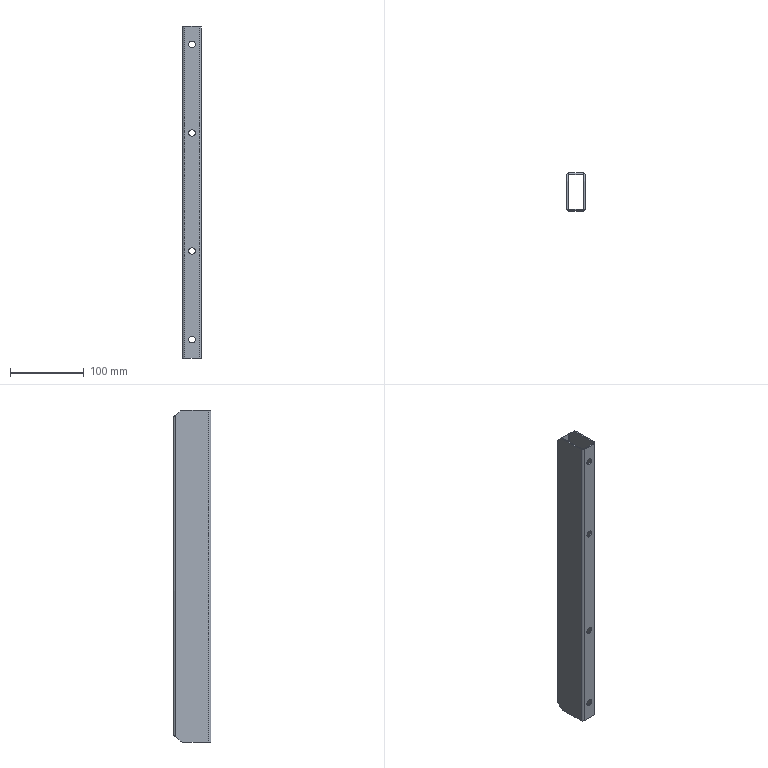Part | STEP file | REFUERZO PLACA BASE POLIPASTO | 1 solid | 40 faces | box 25.4 x 50.8 x 450 mm | volume 118043 mm3 | cylinder 28 | plane 12 | commonest cylinder face diameters 9 x8 14 x8 2.2 x4 6 x4 10 x4
STEP:
#1=CARTESIAN_POINT('',(0.,0.,195.5));
#2=VERTEX_POINT('',#1);
#3=CARTESIAN_POINT('',(0.,0.,204.5));
#4=VERTEX_POINT('',#3);
#5=CARTESIAN_POINT('',(0.,0.,200.));
#6=DIRECTION('',(0.,1.,0.));
#7=DIRECTION('',(-1.,0.,0.));
#8=AXIS2_PLACEMENT_3D('',#5,#6,#7);
#9=CIRCLE('',#8,4.5);
#10=EDGE_CURVE('',#2,#4,#9,.T.);
#11=ORIENTED_EDGE('',*,*,#10,.F.);
#12=CARTESIAN_POINT('',(0.,1.9,195.5));
#13=VERTEX_POINT('',#12);
#14=CARTESIAN_POINT('',(0.,1.9,195.5));
#15=DIRECTION('',(0.,1.,0.));
#16=VECTOR('',#15,1000.);
#17=LINE('',#14,#16);
#18=EDGE_CURVE('',#2,#13,#17,.T.);
#19=ORIENTED_EDGE('',*,*,#18,.T.);
#20=CARTESIAN_POINT('',(0.,1.9,204.5));
#21=VERTEX_POINT('',#20);
#22=CARTESIAN_POINT('',(0.,1.9,200.));
#23=DIRECTION('',(0.,1.,0.));
#24=DIRECTION('',(0.,0.,1.));
#25=AXIS2_PLACEMENT_3D('',#22,#23,#24);
#26=CIRCLE('',#25,4.5);
#27=EDGE_CURVE('',#13,#21,#26,.T.);
#28=ORIENTED_EDGE('',*,*,#27,.T.);
#29=CARTESIAN_POINT('',(0.,1.9,204.5));
#30=DIRECTION('',(0.,1.,0.));
#31=VECTOR('',#30,1000.);
#32=LINE('',#29,#31);
#33=EDGE_CURVE('',#4,#21,#32,.T.);
#34=ORIENTED_EDGE('',*,*,#33,.F.);
#35=EDGE_LOOP('',(#11,#19,#28,#34));
#36=FACE_OUTER_BOUND('',#35,.T.);
#37=CARTESIAN_POINT('',(0.,1.9,200.));
#38=DIRECTION('',(0.,1.,0.));
#39=DIRECTION('',(0.,0.,1.));
#40=AXIS2_PLACEMENT_3D('',#37,#38,#39);
#41=CYLINDRICAL_SURFACE('',#40,4.5);
#42=ADVANCED_FACE('',(#36),#41,.F.);
#43=CARTESIAN_POINT('',(0.,0.,75.5));
#44=VERTEX_POINT('',#43);
#45=CARTESIAN_POINT('',(0.,0.,84.5));
#46=VERTEX_POINT('',#45);
#47=CARTESIAN_POINT('',(0.,0.,80.));
#48=DIRECTION('',(0.,1.,0.));
#49=DIRECTION('',(-1.,0.,0.));
#50=AXIS2_PLACEMENT_3D('',#47,#48,#49);
#51=CIRCLE('',#50,4.5);
#52=EDGE_CURVE('',#44,#46,#51,.T.);
#53=ORIENTED_EDGE('',*,*,#52,.F.);
#54=CARTESIAN_POINT('',(0.,1.9,75.5));
#55=VERTEX_POINT('',#54);
#56=CARTESIAN_POINT('',(0.,1.9,75.5));
#57=DIRECTION('',(0.,1.,0.));
#58=VECTOR('',#57,1000.);
#59=LINE('',#56,#58);
#60=EDGE_CURVE('',#44,#55,#59,.T.);
#61=ORIENTED_EDGE('',*,*,#60,.T.);
#62=CARTESIAN_POINT('',(0.,1.9,84.5));
#63=VERTEX_POINT('',#62);
#64=CARTESIAN_POINT('',(0.,1.9,80.));
#65=DIRECTION('',(0.,1.,0.));
#66=DIRECTION('',(0.,0.,1.));
#67=AXIS2_PLACEMENT_3D('',#64,#65,#66);
#68=CIRCLE('',#67,4.5);
#69=EDGE_CURVE('',#55,#63,#68,.T.);
#70=ORIENTED_EDGE('',*,*,#69,.T.);
#71=CARTESIAN_POINT('',(0.,1.9,84.5));
#72=DIRECTION('',(0.,1.,0.));
#73=VECTOR('',#72,1000.);
#74=LINE('',#71,#73);
#75=EDGE_CURVE('',#46,#63,#74,.T.);
#76=ORIENTED_EDGE('',*,*,#75,.F.);
#77=EDGE_LOOP('',(#53,#61,#70,#76));
#78=FACE_OUTER_BOUND('',#77,.T.);
#79=CARTESIAN_POINT('',(0.,1.9,80.));
#80=DIRECTION('',(0.,1.,0.));
#81=DIRECTION('',(0.,0.,1.));
#82=AXIS2_PLACEMENT_3D('',#79,#80,#81);
#83=CYLINDRICAL_SURFACE('',#82,4.5);
#84=ADVANCED_FACE('',(#78),#83,.F.);
#85=CARTESIAN_POINT('',(0.,0.,-84.5));
#86=VERTEX_POINT('',#85);
#87=CARTESIAN_POINT('',(0.,0.,-75.5));
#88=VERTEX_POINT('',#87);
#89=CARTESIAN_POINT('',(0.,0.,-80.));
#90=DIRECTION('',(0.,1.,0.));
#91=DIRECTION('',(-1.,0.,0.));
#92=AXIS2_PLACEMENT_3D('',#89,#90,#91);
#93=CIRCLE('',#92,4.5);
#94=EDGE_CURVE('',#86,#88,#93,.T.);
#95=ORIENTED_EDGE('',*,*,#94,.F.);
#96=CARTESIAN_POINT('',(0.,1.9,-84.5));
#97=VERTEX_POINT('',#96);
#98=CARTESIAN_POINT('',(0.,1.9,-84.5));
#99=DIRECTION('',(0.,1.,0.));
#100=VECTOR('',#99,1000.);
#101=LINE('',#98,#100);
#102=EDGE_CURVE('',#86,#97,#101,.T.);
#103=ORIENTED_EDGE('',*,*,#102,.T.);
#104=CARTESIAN_POINT('',(0.,1.9,-75.5));
#105=VERTEX_POINT('',#104);
#106=CARTESIAN_POINT('',(0.,1.9,-80.));
#107=DIRECTION('',(0.,1.,0.));
#108=DIRECTION('',(0.,0.,1.));
#109=AXIS2_PLACEMENT_3D('',#106,#107,#108);
#110=CIRCLE('',#109,4.5);
#111=EDGE_CURVE('',#97,#105,#110,.T.);
#112=ORIENTED_EDGE('',*,*,#111,.T.);
#113=CARTESIAN_POINT('',(0.,1.9,-75.5));
#114=DIRECTION('',(0.,1.,0.));
#115=VECTOR('',#114,1000.);
#116=LINE('',#113,#115);
#117=EDGE_CURVE('',#88,#105,#116,.T.);
#118=ORIENTED_EDGE('',*,*,#117,.F.);
#119=EDGE_LOOP('',(#95,#103,#112,#118));
#120=FACE_OUTER_BOUND('',#119,.T.);
#121=CARTESIAN_POINT('',(0.,1.9,-80.));
#122=DIRECTION('',(0.,1.,0.));
#123=DIRECTION('',(0.,0.,1.));
#124=AXIS2_PLACEMENT_3D('',#121,#122,#123);
#125=CYLINDRICAL_SURFACE('',#124,4.5);
#126=ADVANCED_FACE('',(#120),#125,.F.);
#127=CARTESIAN_POINT('',(0.,0.,-204.5));
#128=VERTEX_POINT('',#127);
#129=CARTESIAN_POINT('',(0.,0.,-195.5));
#130=VERTEX_POINT('',#129);
#131=CARTESIAN_POINT('',(0.,0.,-200.));
#132=DIRECTION('',(0.,1.,0.));
#133=DIRECTION('',(-1.,0.,0.));
#134=AXIS2_PLACEMENT_3D('',#131,#132,#133);
#135=CIRCLE('',#134,4.5);
#136=EDGE_CURVE('',#128,#130,#135,.T.);
#137=ORIENTED_EDGE('',*,*,#136,.F.);
#138=CARTESIAN_POINT('',(0.,1.9,-204.5));
#139=VERTEX_POINT('',#138);
#140=CARTESIAN_POINT('',(0.,1.9,-204.5));
#141=DIRECTION('',(0.,1.,0.));
#142=VECTOR('',#141,1000.);
#143=LINE('',#140,#142);
#144=EDGE_CURVE('',#128,#139,#143,.T.);
#145=ORIENTED_EDGE('',*,*,#144,.T.);
#146=CARTESIAN_POINT('',(0.,1.9,-195.5));
#147=VERTEX_POINT('',#146);
#148=CARTESIAN_POINT('',(0.,1.9,-200.));
#149=DIRECTION('',(0.,1.,0.));
#150=DIRECTION('',(0.,0.,1.));
#151=AXIS2_PLACEMENT_3D('',#148,#149,#150);
#152=CIRCLE('',#151,4.5);
#153=EDGE_CURVE('',#139,#147,#152,.T.);
#154=ORIENTED_EDGE('',*,*,#153,.T.);
#155=CARTESIAN_POINT('',(0.,1.9,-195.5));
#156=DIRECTION('',(0.,1.,0.));
#157=VECTOR('',#156,1000.);
#158=LINE('',#155,#157);
#159=EDGE_CURVE('',#130,#147,#158,.T.);
#160=ORIENTED_EDGE('',*,*,#159,.F.);
#161=EDGE_LOOP('',(#137,#145,#154,#160));
#162=FACE_OUTER_BOUND('',#161,.T.);
#163=CARTESIAN_POINT('',(0.,1.9,-200.));
#164=DIRECTION('',(0.,1.,0.));
#165=DIRECTION('',(0.,0.,1.));
#166=AXIS2_PLACEMENT_3D('',#163,#164,#165);
#167=CYLINDRICAL_SURFACE('',#166,4.5);
#168=ADVANCED_FACE('',(#162),#167,.F.);
#169=CARTESIAN_POINT('',(0.,48.9,-193.));
#170=VERTEX_POINT('',#169);
#171=CARTESIAN_POINT('',(0.,48.9,-207.));
#172=VERTEX_POINT('',#171);
#173=CARTESIAN_POINT('',(0.,48.9,-200.));
#174=DIRECTION('',(0.,-1.,0.));
#175=DIRECTION('',(0.,0.,-1.));
#176=AXIS2_PLACEMENT_3D('',#173,#174,#175);
#177=CIRCLE('',#176,7.);
#178=EDGE_CURVE('',#170,#172,#177,.T.);
#179=ORIENTED_EDGE('',*,*,#178,.T.);
#180=CARTESIAN_POINT('',(0.,50.8,-207.));
#181=VERTEX_POINT('',#180);
#182=CARTESIAN_POINT('',(0.,40.8,-207.));
#183=DIRECTION('',(0.,1.,0.));
#184=VECTOR('',#183,1000.);
#185=LINE('',#182,#184);
#186=EDGE_CURVE('',#172,#181,#185,.T.);
#187=ORIENTED_EDGE('',*,*,#186,.T.);
#188=CARTESIAN_POINT('',(0.,50.8,-193.));
#189=VERTEX_POINT('',#188);
#190=CARTESIAN_POINT('',(0.,50.8,-200.));
#191=DIRECTION('',(0.,1.,0.));
#192=DIRECTION('',(0.,0.,1.));
#193=AXIS2_PLACEMENT_3D('',#190,#191,#192);
#194=CIRCLE('',#193,7.);
#195=EDGE_CURVE('',#181,#189,#194,.T.);
#196=ORIENTED_EDGE('',*,*,#195,.T.);
#197=CARTESIAN_POINT('',(0.,40.8,-193.));
#198=DIRECTION('',(0.,1.,0.));
#199=VECTOR('',#198,1000.);
#200=LINE('',#197,#199);
#201=EDGE_CURVE('',#170,#189,#200,.T.);
#202=ORIENTED_EDGE('',*,*,#201,.F.);
#203=EDGE_LOOP('',(#179,#187,#196,#202));
#204=FACE_OUTER_BOUND('',#203,.T.);
#205=CARTESIAN_POINT('',(0.,40.8,-200.));
#206=DIRECTION('',(0.,1.,0.));
#207=DIRECTION('',(0.,0.,1.));
#208=AXIS2_PLACEMENT_3D('',#205,#206,#207);
#209=CYLINDRICAL_SURFACE('',#208,7.);
#210=ADVANCED_FACE('',(#204),#209,.F.);
#211=CARTESIAN_POINT('',(0.,48.9,87.));
#212=VERTEX_POINT('',#211);
#213=CARTESIAN_POINT('',(0.,48.9,73.));
#214=VERTEX_POINT('',#213);
#215=CARTESIAN_POINT('',(0.,48.9,80.));
#216=DIRECTION('',(0.,-1.,0.));
#217=DIRECTION('',(0.,0.,-1.));
#218=AXIS2_PLACEMENT_3D('',#215,#216,#217);
#219=CIRCLE('',#218,7.);
#220=EDGE_CURVE('',#212,#214,#219,.T.);
#221=ORIENTED_EDGE('',*,*,#220,.T.);
#222=CARTESIAN_POINT('',(0.,50.8,73.));
#223=VERTEX_POINT('',#222);
#224=CARTESIAN_POINT('',(0.,40.8,73.));
#225=DIRECTION('',(0.,1.,0.));
#226=VECTOR('',#225,1000.);
#227=LINE('',#224,#226);
#228=EDGE_CURVE('',#214,#223,#227,.T.);
#229=ORIENTED_EDGE('',*,*,#228,.T.);
#230=CARTESIAN_POINT('',(0.,50.8,87.));
#231=VERTEX_POINT('',#230);
#232=CARTESIAN_POINT('',(0.,50.8,80.));
#233=DIRECTION('',(0.,1.,0.));
#234=DIRECTION('',(0.,0.,-1.));
#235=AXIS2_PLACEMENT_3D('',#232,#233,#234);
#236=CIRCLE('',#235,7.);
#237=EDGE_CURVE('',#223,#231,#236,.T.);
#238=ORIENTED_EDGE('',*,*,#237,.T.);
#239=CARTESIAN_POINT('',(0.,40.8,87.));
#240=DIRECTION('',(0.,1.,0.));
#241=VECTOR('',#240,1000.);
#242=LINE('',#239,#241);
#243=EDGE_CURVE('',#212,#231,#242,.T.);
#244=ORIENTED_EDGE('',*,*,#243,.F.);
#245=EDGE_LOOP('',(#221,#229,#238,#244));
#246=FACE_OUTER_BOUND('',#245,.T.);
#247=CARTESIAN_POINT('',(0.,40.8,80.));
#248=DIRECTION('',(0.,1.,0.));
#249=DIRECTION('',(0.,0.,1.));
#250=AXIS2_PLACEMENT_3D('',#247,#248,#249);
#251=CYLINDRICAL_SURFACE('',#250,7.);
#252=ADVANCED_FACE('',(#246),#251,.F.);
#253=CARTESIAN_POINT('',(0.,48.9,-73.));
#254=VERTEX_POINT('',#253);
#255=CARTESIAN_POINT('',(0.,48.9,-87.));
#256=VERTEX_POINT('',#255);
#257=CARTESIAN_POINT('',(0.,48.9,-80.));
#258=DIRECTION('',(0.,-1.,0.));
#259=DIRECTION('',(0.,0.,-1.));
#260=AXIS2_PLACEMENT_3D('',#257,#258,#259);
#261=CIRCLE('',#260,7.);
#262=EDGE_CURVE('',#254,#256,#261,.T.);
#263=ORIENTED_EDGE('',*,*,#262,.T.);
#264=CARTESIAN_POINT('',(0.,50.8,-87.));
#265=VERTEX_POINT('',#264);
#266=CARTESIAN_POINT('',(0.,40.8,-87.));
#267=DIRECTION('',(0.,1.,0.));
#268=VECTOR('',#267,1000.);
#269=LINE('',#266,#268);
#270=EDGE_CURVE('',#256,#265,#269,.T.);
#271=ORIENTED_EDGE('',*,*,#270,.T.);
#272=CARTESIAN_POINT('',(0.,50.8,-73.));
#273=VERTEX_POINT('',#272);
#274=CARTESIAN_POINT('',(0.,50.8,-80.));
#275=DIRECTION('',(0.,1.,0.));
#276=DIRECTION('',(0.,0.,1.));
#277=AXIS2_PLACEMENT_3D('',#274,#275,#276);
#278=CIRCLE('',#277,7.);
#279=EDGE_CURVE('',#265,#273,#278,.T.);
#280=ORIENTED_EDGE('',*,*,#279,.T.);
#281=CARTESIAN_POINT('',(0.,40.8,-73.));
#282=DIRECTION('',(0.,1.,0.));
#283=VECTOR('',#282,1000.);
#284=LINE('',#281,#283);
#285=EDGE_CURVE('',#254,#273,#284,.T.);
#286=ORIENTED_EDGE('',*,*,#285,.F.);
#287=EDGE_LOOP('',(#263,#271,#280,#286));
#288=FACE_OUTER_BOUND('',#287,.T.);
#289=CARTESIAN_POINT('',(0.,40.8,-80.));
#290=DIRECTION('',(0.,1.,0.));
#291=DIRECTION('',(0.,0.,1.));
#292=AXIS2_PLACEMENT_3D('',#289,#290,#291);
#293=CYLINDRICAL_SURFACE('',#292,7.);
#294=ADVANCED_FACE('',(#288),#293,.F.);
#295=CARTESIAN_POINT('',(0.,48.9,207.));
#296=VERTEX_POINT('',#295);
#297=CARTESIAN_POINT('',(0.,48.9,193.));
#298=VERTEX_POINT('',#297);
#299=CARTESIAN_POINT('',(0.,48.9,200.));
#300=DIRECTION('',(0.,-1.,0.));
#301=DIRECTION('',(0.,0.,-1.));
#302=AXIS2_PLACEMENT_3D('',#299,#300,#301);
#303=CIRCLE('',#302,7.);
#304=EDGE_CURVE('',#296,#298,#303,.T.);
#305=ORIENTED_EDGE('',*,*,#304,.T.);
#306=CARTESIAN_POINT('',(0.,50.8,193.));
#307=VERTEX_POINT('',#306);
#308=CARTESIAN_POINT('',(0.,40.8,193.));
#309=DIRECTION('',(0.,1.,0.));
#310=VECTOR('',#309,1000.);
#311=LINE('',#308,#310);
#312=EDGE_CURVE('',#298,#307,#311,.T.);
#313=ORIENTED_EDGE('',*,*,#312,.T.);
#314=CARTESIAN_POINT('',(0.,50.8,207.));
#315=VERTEX_POINT('',#314);
#316=CARTESIAN_POINT('',(0.,50.8,200.));
#317=DIRECTION('',(0.,1.,0.));
#318=DIRECTION('',(0.,0.,-1.));
#319=AXIS2_PLACEMENT_3D('',#316,#317,#318);
#320=CIRCLE('',#319,7.);
#321=EDGE_CURVE('',#307,#315,#320,.T.);
#322=ORIENTED_EDGE('',*,*,#321,.T.);
#323=CARTESIAN_POINT('',(0.,40.8,207.));
#324=DIRECTION('',(0.,1.,0.));
#325=VECTOR('',#324,1000.);
#326=LINE('',#323,#325);
#327=EDGE_CURVE('',#296,#315,#326,.T.);
#328=ORIENTED_EDGE('',*,*,#327,.F.);
#329=EDGE_LOOP('',(#305,#313,#322,#328));
#330=FACE_OUTER_BOUND('',#329,.T.);
#331=CARTESIAN_POINT('',(0.,40.8,200.));
#332=DIRECTION('',(0.,1.,0.));
#333=DIRECTION('',(0.,0.,1.));
#334=AXIS2_PLACEMENT_3D('',#331,#332,#333);
#335=CYLINDRICAL_SURFACE('',#334,7.);
#336=ADVANCED_FACE('',(#330),#335,.F.);
#337=CARTESIAN_POINT('',(-10.8,38.041,225.));
#338=VERTEX_POINT('',#337);
#339=CARTESIAN_POINT('',(-10.8,3.,225.));
#340=VERTEX_POINT('',#339);
#341=CARTESIAN_POINT('',(-10.8,47.8,225.));
#342=DIRECTION('',(0.,-1.,0.));
#343=VECTOR('',#342,1000.);
#344=LINE('',#341,#343);
#345=EDGE_CURVE('',#338,#340,#344,.T.);
#346=ORIENTED_EDGE('',*,*,#345,.F.);
#347=CARTESIAN_POINT('',(-12.7,38.041,225.));
#348=VERTEX_POINT('',#347);
#349=CARTESIAN_POINT('',(-12.7,38.041,225.));
#350=DIRECTION('',(-1.,0.,0.));
#351=VECTOR('',#350,1000.);
#352=LINE('',#349,#351);
#353=EDGE_CURVE('',#338,#348,#352,.T.);
#354=ORIENTED_EDGE('',*,*,#353,.T.);
#355=CARTESIAN_POINT('',(-12.7,3.,225.));
#356=VERTEX_POINT('',#355);
#357=CARTESIAN_POINT('',(-12.7,47.8,225.));
#358=DIRECTION('',(0.,-1.,0.));
#359=VECTOR('',#358,1000.);
#360=LINE('',#357,#359);
#361=EDGE_CURVE('',#348,#356,#360,.T.);
#362=ORIENTED_EDGE('',*,*,#361,.T.);
#363=CARTESIAN_POINT('',(-9.7,0.,225.));
#364=VERTEX_POINT('',#363);
#365=CARTESIAN_POINT('',(-9.7,3.,225.));
#366=DIRECTION('',(0.,0.,1.));
#367=DIRECTION('',(1.,0.,0.));
#368=AXIS2_PLACEMENT_3D('',#365,#366,#367);
#369=CIRCLE('',#368,3.);
#370=EDGE_CURVE('',#356,#364,#369,.T.);
#371=ORIENTED_EDGE('',*,*,#370,.T.);
#372=CARTESIAN_POINT('',(9.7,0.,225.));
#373=VERTEX_POINT('',#372);
#374=CARTESIAN_POINT('',(-9.7,0.,225.));
#375=DIRECTION('',(1.,0.,0.));
#376=VECTOR('',#375,1000.);
#377=LINE('',#374,#376);
#378=EDGE_CURVE('',#364,#373,#377,.T.);
#379=ORIENTED_EDGE('',*,*,#378,.T.);
#380=CARTESIAN_POINT('',(12.7,3.,225.));
#381=VERTEX_POINT('',#380);
#382=CARTESIAN_POINT('',(9.7,3.,225.));
#383=DIRECTION('',(0.,0.,1.));
#384=DIRECTION('',(1.,0.,0.));
#385=AXIS2_PLACEMENT_3D('',#382,#383,#384);
#386=CIRCLE('',#385,3.);
#387=EDGE_CURVE('',#373,#381,#386,.T.);
#388=ORIENTED_EDGE('',*,*,#387,.T.);
#389=CARTESIAN_POINT('',(12.7,38.041,225.));
#390=VERTEX_POINT('',#389);
#391=CARTESIAN_POINT('',(12.7,47.8,225.));
#392=DIRECTION('',(0.,1.,0.));
#393=VECTOR('',#392,1000.);
#394=LINE('',#391,#393);
#395=EDGE_CURVE('',#381,#390,#394,.T.);
#396=ORIENTED_EDGE('',*,*,#395,.T.);
#397=CARTESIAN_POINT('',(10.8,38.041,225.));
#398=VERTEX_POINT('',#397);
#399=CARTESIAN_POINT('',(10.8,38.041,225.));
#400=DIRECTION('',(-1.,0.,0.));
#401=VECTOR('',#400,1000.);
#402=LINE('',#399,#401);
#403=EDGE_CURVE('',#390,#398,#402,.T.);
#404=ORIENTED_EDGE('',*,*,#403,.T.);
#405=CARTESIAN_POINT('',(10.8,3.,225.));
#406=VERTEX_POINT('',#405);
#407=CARTESIAN_POINT('',(10.8,47.8,225.));
#408=DIRECTION('',(0.,1.,0.));
#409=VECTOR('',#408,1000.);
#410=LINE('',#407,#409);
#411=EDGE_CURVE('',#406,#398,#410,.T.);
#412=ORIENTED_EDGE('',*,*,#411,.F.);
#413=CARTESIAN_POINT('',(9.7,1.9,225.));
#414=VERTEX_POINT('',#413);
#415=CARTESIAN_POINT('',(9.7,3.,225.));
#416=DIRECTION('',(0.,0.,1.));
#417=DIRECTION('',(-1.,0.,0.));
#418=AXIS2_PLACEMENT_3D('',#415,#416,#417);
#419=CIRCLE('',#418,1.1);
#420=EDGE_CURVE('',#414,#406,#419,.T.);
#421=ORIENTED_EDGE('',*,*,#420,.F.);
#422=CARTESIAN_POINT('',(-9.7,1.9,225.));
#423=VERTEX_POINT('',#422);
#424=CARTESIAN_POINT('',(9.7,1.9,225.));
#425=DIRECTION('',(1.,0.,0.));
#426=VECTOR('',#425,1000.);
#427=LINE('',#424,#426);
#428=EDGE_CURVE('',#423,#414,#427,.T.);
#429=ORIENTED_EDGE('',*,*,#428,.F.);
#430=CARTESIAN_POINT('',(-9.7,3.,225.));
#431=DIRECTION('',(0.,0.,1.));
#432=DIRECTION('',(-1.,0.,0.));
#433=AXIS2_PLACEMENT_3D('',#430,#431,#432);
#434=CIRCLE('',#433,1.1);
#435=EDGE_CURVE('',#340,#423,#434,.T.);
#436=ORIENTED_EDGE('',*,*,#435,.F.);
#437=EDGE_LOOP('',(#346,#354,#362,#371,#379,#388,#396,#404,#412,#421,#429,#436));
#438=FACE_OUTER_BOUND('',#437,.T.);
#439=CARTESIAN_POINT('',(9.7,47.8,225.));
#440=DIRECTION('',(0.,0.,1.));
#441=DIRECTION('',(1.,0.,0.));
#442=AXIS2_PLACEMENT_3D('',#439,#440,#441);
#443=PLANE('',#442);
#444=ADVANCED_FACE('',(#438),#443,.T.);
#445=CARTESIAN_POINT('',(-12.7,38.041,-225.));
#446=VERTEX_POINT('',#445);
#447=CARTESIAN_POINT('',(-12.7,3.,-225.));
#448=VERTEX_POINT('',#447);
#449=CARTESIAN_POINT('',(-12.7,47.8,-225.));
#450=DIRECTION('',(0.,-1.,0.));
#451=VECTOR('',#450,1000.);
#452=LINE('',#449,#451);
#453=EDGE_CURVE('',#446,#448,#452,.T.);
#454=ORIENTED_EDGE('',*,*,#453,.F.);
#455=CARTESIAN_POINT('',(-10.8,38.041,-225.));
#456=VERTEX_POINT('',#455);
#457=CARTESIAN_POINT('',(9.7,38.041,-225.));
#458=DIRECTION('',(1.,0.,0.));
#459=VECTOR('',#458,1000.);
#460=LINE('',#457,#459);
#461=EDGE_CURVE('',#446,#456,#460,.T.);
#462=ORIENTED_EDGE('',*,*,#461,.T.);
#463=CARTESIAN_POINT('',(-10.8,3.,-225.));
#464=VERTEX_POINT('',#463);
#465=CARTESIAN_POINT('',(-10.8,47.8,-225.));
#466=DIRECTION('',(0.,-1.,0.));
#467=VECTOR('',#466,1000.);
#468=LINE('',#465,#467);
#469=EDGE_CURVE('',#456,#464,#468,.T.);
#470=ORIENTED_EDGE('',*,*,#469,.T.);
#471=CARTESIAN_POINT('',(-9.7,1.9,-225.));
#472=VERTEX_POINT('',#471);
#473=CARTESIAN_POINT('',(-9.7,3.,-225.));
#474=DIRECTION('',(0.,0.,1.));
#475=DIRECTION('',(-1.,0.,0.));
#476=AXIS2_PLACEMENT_3D('',#473,#474,#475);
#477=CIRCLE('',#476,1.1);
#478=EDGE_CURVE('',#464,#472,#477,.T.);
#479=ORIENTED_EDGE('',*,*,#478,.T.);
#480=CARTESIAN_POINT('',(9.7,1.9,-225.));
#481=VERTEX_POINT('',#480);
#482=CARTESIAN_POINT('',(9.7,1.9,-225.));
#483=DIRECTION('',(1.,0.,0.));
#484=VECTOR('',#483,1000.);
#485=LINE('',#482,#484);
#486=EDGE_CURVE('',#472,#481,#485,.T.);
#487=ORIENTED_EDGE('',*,*,#486,.T.);
#488=CARTESIAN_POINT('',(10.8,3.,-225.));
#489=VERTEX_POINT('',#488);
#490=CARTESIAN_POINT('',(9.7,3.,-225.));
#491=DIRECTION('',(0.,0.,1.));
#492=DIRECTION('',(-1.,0.,0.));
#493=AXIS2_PLACEMENT_3D('',#490,#491,#492);
#494=CIRCLE('',#493,1.1);
#495=EDGE_CURVE('',#481,#489,#494,.T.);
#496=ORIENTED_EDGE('',*,*,#495,.T.);
#497=CARTESIAN_POINT('',(10.8,38.041,-225.));
#498=VERTEX_POINT('',#497);
#499=CARTESIAN_POINT('',(10.8,47.8,-225.));
#500=DIRECTION('',(0.,1.,0.));
#501=VECTOR('',#500,1000.);
#502=LINE('',#499,#501);
#503=EDGE_CURVE('',#489,#498,#502,.T.);
#504=ORIENTED_EDGE('',*,*,#503,.T.);
#505=CARTESIAN_POINT('',(12.7,38.041,-225.));
#506=VERTEX_POINT('',#505);
#507=CARTESIAN_POINT('',(9.7,38.041,-225.));
#508=DIRECTION('',(1.,0.,0.));
#509=VECTOR('',#508,1000.);
#510=LINE('',#507,#509);
#511=EDGE_CURVE('',#498,#506,#510,.T.);
#512=ORIENTED_EDGE('',*,*,#511,.T.);
#513=CARTESIAN_POINT('',(12.7,3.,-225.));
#514=VERTEX_POINT('',#513);
#515=CARTESIAN_POINT('',(12.7,47.8,-225.));
#516=DIRECTION('',(0.,1.,0.));
#517=VECTOR('',#516,1000.);
#518=LINE('',#515,#517);
#519=EDGE_CURVE('',#514,#506,#518,.T.);
#520=ORIENTED_EDGE('',*,*,#519,.F.);
#521=CARTESIAN_POINT('',(9.7,0.,-225.));
#522=VERTEX_POINT('',#521);
#523=CARTESIAN_POINT('',(9.7,3.,-225.));
#524=DIRECTION('',(0.,0.,1.));
#525=DIRECTION('',(1.,0.,0.));
#526=AXIS2_PLACEMENT_3D('',#523,#524,#525);
#527=CIRCLE('',#526,3.);
#528=EDGE_CURVE('',#522,#514,#527,.T.);
#529=ORIENTED_EDGE('',*,*,#528,.F.);
#530=CARTESIAN_POINT('',(-9.7,0.,-225.));
#531=VERTEX_POINT('',#530);
#532=CARTESIAN_POINT('',(-9.7,0.,-225.));
#533=DIRECTION('',(1.,0.,0.));
#534=VECTOR('',#533,1000.);
#535=LINE('',#532,#534);
#536=EDGE_CURVE('',#531,#522,#535,.T.);
#537=ORIENTED_EDGE('',*,*,#536,.F.);
#538=CARTESIAN_POINT('',(-9.7,3.,-225.));
#539=DIRECTION('',(0.,0.,1.));
#540=DIRECTION('',(1.,0.,0.));
#541=AXIS2_PLACEMENT_3D('',#538,#539,#540);
#542=CIRCLE('',#541,3.);
#543=EDGE_CURVE('',#448,#531,#542,.T.);
#544=ORIENTED_EDGE('',*,*,#543,.F.);
#545=EDGE_LOOP('',(#454,#462,#470,#479,#487,#496,#504,#512,#520,#529,#537,#544));
#546=FACE_OUTER_BOUND('',#545,.T.);
#547=CARTESIAN_POINT('',(9.7,47.8,-225.));
#548=DIRECTION('',(0.,0.,1.));
#549=DIRECTION('',(1.,0.,0.));
#550=AXIS2_PLACEMENT_3D('',#547,#548,#549);
#551=PLANE('',#550);
#552=ADVANCED_FACE('',(#546),#551,.F.);
#553=CARTESIAN_POINT('',(9.7,50.8,215.));
#554=VERTEX_POINT('',#553);
#555=CARTESIAN_POINT('',(9.7,50.8,-215.));
#556=VERTEX_POINT('',#555);
#557=CARTESIAN_POINT('',(9.7,50.8,225.));
#558=DIRECTION('',(0.,0.,-1.));
#559=VECTOR('',#558,1000.);
#560=LINE('',#557,#559);
#561=EDGE_CURVE('',#554,#556,#560,.T.);
#562=ORIENTED_EDGE('',*,*,#561,.F.);
#563=CARTESIAN_POINT('',(12.7,47.8,217.778));
#564=VERTEX_POINT('',#563);
#565=CARTESIAN_POINT('',(9.7,50.8,215.));
#566=CARTESIAN_POINT('',(11.457,50.8,215.));
#567=CARTESIAN_POINT('',(12.7,49.557,216.151));
#568=CARTESIAN_POINT('',(12.7,47.8,217.778));
#569=(BOUNDED_CURVE()B_SPLINE_CURVE(3,(#565,#566,#567,#568),.UNSPECIFIED.,.F.,.F.)B_SPLINE_CURVE_WITH_KNOTS((4,4),(0.,1.571),.UNSPECIFIED.)CURVE()GEOMETRIC_REPRESENTATION_ITEM()RATIONAL_B_SPLINE_CURVE((1.,0.8047,0.8047,1.))REPRESENTATION_ITEM(''));
#570=EDGE_CURVE('',#554,#564,#569,.T.);
#571=ORIENTED_EDGE('',*,*,#570,.T.);
#572=CARTESIAN_POINT('',(12.7,47.8,-217.778));
#573=VERTEX_POINT('',#572);
#574=CARTESIAN_POINT('',(12.7,47.8,225.));
#575=DIRECTION('',(0.,0.,-1.));
#576=VECTOR('',#575,1000.);
#577=LINE('',#574,#576);
#578=EDGE_CURVE('',#564,#573,#577,.T.);
#579=ORIENTED_EDGE('',*,*,#578,.T.);
#580=CARTESIAN_POINT('',(12.7,47.8,-217.778));
#581=CARTESIAN_POINT('',(12.7,49.557,-216.151));
#582=CARTESIAN_POINT('',(11.457,50.8,-215.));
#583=CARTESIAN_POINT('',(9.7,50.8,-215.));
#584=(BOUNDED_CURVE()B_SPLINE_CURVE(3,(#580,#581,#582,#583),.UNSPECIFIED.,.F.,.F.)B_SPLINE_CURVE_WITH_KNOTS((4,4),(1.571,3.142),.UNSPECIFIED.)CURVE()GEOMETRIC_REPRESENTATION_ITEM()RATIONAL_B_SPLINE_CURVE((1.,0.8047,0.8047,1.))REPRESENTATION_ITEM(''));
#585=EDGE_CURVE('',#573,#556,#584,.T.);
#586=ORIENTED_EDGE('',*,*,#585,.T.);
#587=EDGE_LOOP('',(#562,#571,#579,#586));
#588=FACE_OUTER_BOUND('',#587,.T.);
#589=CARTESIAN_POINT('',(9.7,47.8,225.));
#590=DIRECTION('',(0.,0.,-1.));
#591=DIRECTION('',(-1.,0.,0.));
#592=AXIS2_PLACEMENT_3D('',#589,#590,#591);
#593=CYLINDRICAL_SURFACE('',#592,3.);
#594=ADVANCED_FACE('',(#588),#593,.T.);
#595=CARTESIAN_POINT('',(0.,50.8,-200.));
#596=DIRECTION('',(0.,1.,0.));
#597=DIRECTION('',(0.,0.,1.));
#598=AXIS2_PLACEMENT_3D('',#595,#596,#597);
#599=CIRCLE('',#598,7.);
#600=EDGE_CURVE('',#189,#181,#599,.T.);
#601=ORIENTED_EDGE('',*,*,#600,.F.);
#602=ORIENTED_EDGE('',*,*,#195,.F.);
#603=EDGE_LOOP('',(#601,#602));
#604=FACE_BOUND('',#603,.T.);
#605=CARTESIAN_POINT('',(0.,50.8,80.));
#606=DIRECTION('',(0.,1.,0.));
#607=DIRECTION('',(0.,0.,-1.));
#608=AXIS2_PLACEMENT_3D('',#605,#606,#607);
#609=CIRCLE('',#608,7.);
#610=EDGE_CURVE('',#231,#223,#609,.T.);
#611=ORIENTED_EDGE('',*,*,#610,.F.);
#612=ORIENTED_EDGE('',*,*,#237,.F.);
#613=EDGE_LOOP('',(#611,#612));
#614=FACE_BOUND('',#613,.T.);
#615=CARTESIAN_POINT('',(0.,50.8,-80.));
#616=DIRECTION('',(0.,1.,0.));
#617=DIRECTION('',(0.,0.,1.));
#618=AXIS2_PLACEMENT_3D('',#615,#616,#617);
#619=CIRCLE('',#618,7.);
#620=EDGE_CURVE('',#273,#265,#619,.T.);
#621=ORIENTED_EDGE('',*,*,#620,.F.);
#622=ORIENTED_EDGE('',*,*,#279,.F.);
#623=EDGE_LOOP('',(#621,#622));
#624=FACE_BOUND('',#623,.T.);
#625=CARTESIAN_POINT('',(0.,50.8,200.));
#626=DIRECTION('',(0.,1.,0.));
#627=DIRECTION('',(0.,0.,-1.));
#628=AXIS2_PLACEMENT_3D('',#625,#626,#627);
#629=CIRCLE('',#628,7.);
#630=EDGE_CURVE('',#315,#307,#629,.T.);
#631=ORIENTED_EDGE('',*,*,#630,.F.);
#632=ORIENTED_EDGE('',*,*,#321,.F.);
#633=EDGE_LOOP('',(#631,#632));
#634=FACE_BOUND('',#633,.T.);
#635=CARTESIAN_POINT('',(-9.7,50.8,215.));
#636=VERTEX_POINT('',#635);
#637=CARTESIAN_POINT('',(-9.7,50.8,-215.));
#638=VERTEX_POINT('',#637);
#639=CARTESIAN_POINT('',(-9.7,50.8,225.));
#640=DIRECTION('',(0.,0.,-1.));
#641=VECTOR('',#640,1000.);
#642=LINE('',#639,#641);
#643=EDGE_CURVE('',#636,#638,#642,.T.);
#644=ORIENTED_EDGE('',*,*,#643,.F.);
#645=CARTESIAN_POINT('',(-12.7,50.8,215.));
#646=DIRECTION('',(1.,0.,0.));
#647=VECTOR('',#646,1000.);
#648=LINE('',#645,#647);
#649=EDGE_CURVE('',#636,#554,#648,.T.);
#650=ORIENTED_EDGE('',*,*,#649,.T.);
#651=ORIENTED_EDGE('',*,*,#561,.T.);
#652=CARTESIAN_POINT('',(-12.7,50.8,-215.));
#653=DIRECTION('',(1.,0.,0.));
#654=VECTOR('',#653,1000.);
#655=LINE('',#652,#654);
#656=EDGE_CURVE('',#638,#556,#655,.T.);
#657=ORIENTED_EDGE('',*,*,#656,.F.);
#658=EDGE_LOOP('',(#644,#650,#651,#657));
#659=FACE_OUTER_BOUND('',#658,.T.);
#660=CARTESIAN_POINT('',(-9.7,50.8,225.));
#661=DIRECTION('',(0.,-1.,0.));
#662=DIRECTION('',(0.,0.,-1.));
#663=AXIS2_PLACEMENT_3D('',#660,#661,#662);
#664=PLANE('',#663);
#665=ADVANCED_FACE('',(#604,#614,#624,#634,#659),#664,.F.);
#666=CARTESIAN_POINT('',(-12.7,47.8,217.778));
#667=VERTEX_POINT('',#666);
#668=CARTESIAN_POINT('',(-12.7,47.8,-217.778));
#669=VERTEX_POINT('',#668);
#670=CARTESIAN_POINT('',(-12.7,47.8,225.));
#671=DIRECTION('',(0.,0.,-1.));
#672=VECTOR('',#671,1000.);
#673=LINE('',#670,#672);
#674=EDGE_CURVE('',#667,#669,#673,.T.);
#675=ORIENTED_EDGE('',*,*,#674,.F.);
#676=CARTESIAN_POINT('',(-12.7,47.8,217.778));
#677=CARTESIAN_POINT('',(-12.7,49.557,216.151));
#678=CARTESIAN_POINT('',(-11.457,50.8,215.));
#679=CARTESIAN_POINT('',(-9.7,50.8,215.));
#680=(BOUNDED_CURVE()B_SPLINE_CURVE(3,(#676,#677,#678,#679),.UNSPECIFIED.,.F.,.F.)B_SPLINE_CURVE_WITH_KNOTS((4,4),(4.712,6.283),.UNSPECIFIED.)CURVE()GEOMETRIC_REPRESENTATION_ITEM()RATIONAL_B_SPLINE_CURVE((1.,0.8047,0.8047,1.))REPRESENTATION_ITEM(''));
#681=EDGE_CURVE('',#667,#636,#680,.T.);
#682=ORIENTED_EDGE('',*,*,#681,.T.);
#683=ORIENTED_EDGE('',*,*,#643,.T.);
#684=CARTESIAN_POINT('',(-9.7,50.8,-215.));
#685=CARTESIAN_POINT('',(-11.457,50.8,-215.));
#686=CARTESIAN_POINT('',(-12.7,49.557,-216.151));
#687=CARTESIAN_POINT('',(-12.7,47.8,-217.778));
#688=(BOUNDED_CURVE()B_SPLINE_CURVE(3,(#684,#685,#686,#687),.UNSPECIFIED.,.F.,.F.)B_SPLINE_CURVE_WITH_KNOTS((4,4),(3.142,4.712),.UNSPECIFIED.)CURVE()GEOMETRIC_REPRESENTATION_ITEM()RATIONAL_B_SPLINE_CURVE((1.,0.8047,0.8047,1.))REPRESENTATION_ITEM(''));
#689=EDGE_CURVE('',#638,#669,#688,.T.);
#690=ORIENTED_EDGE('',*,*,#689,.T.);
#691=EDGE_LOOP('',(#675,#682,#683,#690));
#692=FACE_OUTER_BOUND('',#691,.T.);
#693=CARTESIAN_POINT('',(-9.7,47.8,225.));
#694=DIRECTION('',(0.,0.,-1.));
#695=DIRECTION('',(-1.,0.,0.));
#696=AXIS2_PLACEMENT_3D('',#693,#694,#695);
#697=CYLINDRICAL_SURFACE('',#696,3.);
#698=ADVANCED_FACE('',(#692),#697,.T.);
#699=CARTESIAN_POINT('',(-12.7,41.438,-223.669));
#700=VERTEX_POINT('',#699);
#701=CARTESIAN_POINT('',(-12.7,50.8,-215.));
#702=DIRECTION('',(0.,-0.7338,-0.6794));
#703=VECTOR('',#702,1000.);
#704=LINE('',#701,#703);
#705=EDGE_CURVE('',#669,#700,#704,.T.);
#706=ORIENTED_EDGE('',*,*,#705,.T.);
#707=CARTESIAN_POINT('',(-12.7,38.041,-220.));
#708=DIRECTION('',(-1.,0.,0.));
#709=DIRECTION('',(0.,1.,0.));
#710=AXIS2_PLACEMENT_3D('',#707,#708,#709);
#711=CIRCLE('',#710,5.);
#712=EDGE_CURVE('',#700,#446,#711,.T.);
#713=ORIENTED_EDGE('',*,*,#712,.T.);
#714=ORIENTED_EDGE('',*,*,#453,.T.);
#715=CARTESIAN_POINT('',(-12.7,3.,225.));
#716=DIRECTION('',(0.,0.,-1.));
#717=VECTOR('',#716,1000.);
#718=LINE('',#715,#717);
#719=EDGE_CURVE('',#356,#448,#718,.T.);
#720=ORIENTED_EDGE('',*,*,#719,.F.);
#721=ORIENTED_EDGE('',*,*,#361,.F.);
#722=CARTESIAN_POINT('',(-12.7,41.438,223.669));
#723=VERTEX_POINT('',#722);
#724=CARTESIAN_POINT('',(-12.7,38.041,220.));
#725=DIRECTION('',(-1.,0.,0.));
#726=DIRECTION('',(0.,1.,0.));
#727=AXIS2_PLACEMENT_3D('',#724,#725,#726);
#728=CIRCLE('',#727,5.);
#729=EDGE_CURVE('',#348,#723,#728,.T.);
#730=ORIENTED_EDGE('',*,*,#729,.T.);
#731=CARTESIAN_POINT('',(-12.7,50.8,215.));
#732=DIRECTION('',(0.,0.7338,-0.6794));
#733=VECTOR('',#732,1000.);
#734=LINE('',#731,#733);
#735=EDGE_CURVE('',#723,#667,#734,.T.);
#736=ORIENTED_EDGE('',*,*,#735,.T.);
#737=ORIENTED_EDGE('',*,*,#674,.T.);
#738=EDGE_LOOP('',(#706,#713,#714,#720,#721,#730,#736,#737));
#739=FACE_OUTER_BOUND('',#738,.T.);
#740=CARTESIAN_POINT('',(-12.7,47.8,225.));
#741=DIRECTION('',(1.,0.,0.));
#742=DIRECTION('',(0.,1.,0.));
#743=AXIS2_PLACEMENT_3D('',#740,#741,#742);
#744=PLANE('',#743);
#745=ADVANCED_FACE('',(#739),#744,.F.);
#746=ORIENTED_EDGE('',*,*,#543,.T.);
#747=CARTESIAN_POINT('',(-9.7,0.,225.));
#748=DIRECTION('',(0.,0.,-1.));
#749=VECTOR('',#748,1000.);
#750=LINE('',#747,#749);
#751=EDGE_CURVE('',#364,#531,#750,.T.);
#752=ORIENTED_EDGE('',*,*,#751,.F.);
#753=ORIENTED_EDGE('',*,*,#370,.F.);
#754=ORIENTED_EDGE('',*,*,#719,.T.);
#755=EDGE_LOOP('',(#746,#752,#753,#754));
#756=FACE_OUTER_BOUND('',#755,.T.);
#757=CARTESIAN_POINT('',(-9.7,3.,225.));
#758=DIRECTION('',(0.,0.,-1.));
#759=DIRECTION('',(-1.,0.,0.));
#760=AXIS2_PLACEMENT_3D('',#757,#758,#759);
#761=CYLINDRICAL_SURFACE('',#760,3.);
#762=ADVANCED_FACE('',(#756),#761,.T.);
#763=CARTESIAN_POINT('',(0.,0.,200.));
#764=DIRECTION('',(0.,1.,0.));
#765=DIRECTION('',(-1.,0.,0.));
#766=AXIS2_PLACEMENT_3D('',#763,#764,#765);
#767=CIRCLE('',#766,4.5);
#768=EDGE_CURVE('',#4,#2,#767,.T.);
#769=ORIENTED_EDGE('',*,*,#768,.T.);
#770=ORIENTED_EDGE('',*,*,#10,.T.);
#771=EDGE_LOOP('',(#769,#770));
#772=FACE_BOUND('',#771,.T.);
#773=CARTESIAN_POINT('',(0.,0.,80.));
#774=DIRECTION('',(0.,1.,0.));
#775=DIRECTION('',(-1.,0.,0.));
#776=AXIS2_PLACEMENT_3D('',#773,#774,#775);
#777=CIRCLE('',#776,4.5);
#778=EDGE_CURVE('',#46,#44,#777,.T.);
#779=ORIENTED_EDGE('',*,*,#778,.T.);
#780=ORIENTED_EDGE('',*,*,#52,.T.);
#781=EDGE_LOOP('',(#779,#780));
#782=FACE_BOUND('',#781,.T.);
#783=CARTESIAN_POINT('',(0.,0.,-80.));
#784=DIRECTION('',(0.,1.,0.));
#785=DIRECTION('',(-1.,0.,0.));
#786=AXIS2_PLACEMENT_3D('',#783,#784,#785);
#787=CIRCLE('',#786,4.5);
#788=EDGE_CURVE('',#88,#86,#787,.T.);
#789=ORIENTED_EDGE('',*,*,#788,.T.);
#790=ORIENTED_EDGE('',*,*,#94,.T.);
#791=EDGE_LOOP('',(#789,#790));
#792=FACE_BOUND('',#791,.T.);
#793=CARTESIAN_POINT('',(0.,0.,-200.));
#794=DIRECTION('',(0.,1.,0.));
#795=DIRECTION('',(-1.,0.,0.));
#796=AXIS2_PLACEMENT_3D('',#793,#794,#795);
#797=CIRCLE('',#796,4.5);
#798=EDGE_CURVE('',#130,#128,#797,.T.);
#799=ORIENTED_EDGE('',*,*,#798,.T.);
#800=ORIENTED_EDGE('',*,*,#136,.T.);
#801=EDGE_LOOP('',(#799,#800));
#802=FACE_BOUND('',#801,.T.);
#803=ORIENTED_EDGE('',*,*,#536,.T.);
#804=CARTESIAN_POINT('',(9.7,0.,225.));
#805=DIRECTION('',(0.,0.,-1.));
#806=VECTOR('',#805,1000.);
#807=LINE('',#804,#806);
#808=EDGE_CURVE('',#373,#522,#807,.T.);
#809=ORIENTED_EDGE('',*,*,#808,.F.);
#810=ORIENTED_EDGE('',*,*,#378,.F.);
#811=ORIENTED_EDGE('',*,*,#751,.T.);
#812=EDGE_LOOP('',(#803,#809,#810,#811));
#813=FACE_OUTER_BOUND('',#812,.T.);
#814=CARTESIAN_POINT('',(-9.7,0.,225.));
#815=DIRECTION('',(0.,1.,0.));
#816=DIRECTION('',(-1.,0.,0.));
#817=AXIS2_PLACEMENT_3D('',#814,#815,#816);
#818=PLANE('',#817);
#819=ADVANCED_FACE('',(#772,#782,#792,#802,#813),#818,.F.);
#820=ORIENTED_EDGE('',*,*,#528,.T.);
#821=CARTESIAN_POINT('',(12.7,3.,225.));
#822=DIRECTION('',(0.,0.,-1.));
#823=VECTOR('',#822,1000.);
#824=LINE('',#821,#823);
#825=EDGE_CURVE('',#381,#514,#824,.T.);
#826=ORIENTED_EDGE('',*,*,#825,.F.);
#827=ORIENTED_EDGE('',*,*,#387,.F.);
#828=ORIENTED_EDGE('',*,*,#808,.T.);
#829=EDGE_LOOP('',(#820,#826,#827,#828));
#830=FACE_OUTER_BOUND('',#829,.T.);
#831=CARTESIAN_POINT('',(9.7,3.,225.));
#832=DIRECTION('',(0.,0.,-1.));
#833=DIRECTION('',(-1.,0.,0.));
#834=AXIS2_PLACEMENT_3D('',#831,#832,#833);
#835=CYLINDRICAL_SURFACE('',#834,3.);
#836=ADVANCED_FACE('',(#830),#835,.T.);
#837=ORIENTED_EDGE('',*,*,#519,.T.);
#838=CARTESIAN_POINT('',(12.7,41.438,-223.669));
#839=VERTEX_POINT('',#838);
#840=CARTESIAN_POINT('',(12.7,38.041,-220.));
#841=DIRECTION('',(1.,0.,0.));
#842=DIRECTION('',(0.,-1.,0.));
#843=AXIS2_PLACEMENT_3D('',#840,#841,#842);
#844=CIRCLE('',#843,5.);
#845=EDGE_CURVE('',#506,#839,#844,.T.);
#846=ORIENTED_EDGE('',*,*,#845,.T.);
#847=CARTESIAN_POINT('',(12.7,268.535,-13.394));
#848=DIRECTION('',(0.,0.7338,0.6794));
#849=VECTOR('',#848,1000.);
#850=LINE('',#847,#849);
#851=EDGE_CURVE('',#839,#573,#850,.T.);
#852=ORIENTED_EDGE('',*,*,#851,.T.);
#853=ORIENTED_EDGE('',*,*,#578,.F.);
#854=CARTESIAN_POINT('',(12.7,41.438,223.669));
#855=VERTEX_POINT('',#854);
#856=CARTESIAN_POINT('',(12.7,44.2,221.112));
#857=DIRECTION('',(0.,-0.7338,0.6794));
#858=VECTOR('',#857,1000.);
#859=LINE('',#856,#858);
#860=EDGE_CURVE('',#564,#855,#859,.T.);
#861=ORIENTED_EDGE('',*,*,#860,.T.);
#862=CARTESIAN_POINT('',(12.7,38.041,220.));
#863=DIRECTION('',(1.,0.,0.));
#864=DIRECTION('',(0.,-1.,0.));
#865=AXIS2_PLACEMENT_3D('',#862,#863,#864);
#866=CIRCLE('',#865,5.);
#867=EDGE_CURVE('',#855,#390,#866,.T.);
#868=ORIENTED_EDGE('',*,*,#867,.T.);
#869=ORIENTED_EDGE('',*,*,#395,.F.);
#870=ORIENTED_EDGE('',*,*,#825,.T.);
#871=EDGE_LOOP('',(#837,#846,#852,#853,#861,#868,#869,#870));
#872=FACE_OUTER_BOUND('',#871,.T.);
#873=CARTESIAN_POINT('',(12.7,47.8,225.));
#874=DIRECTION('',(-1.,0.,0.));
#875=DIRECTION('',(0.,-1.,0.));
#876=AXIS2_PLACEMENT_3D('',#873,#874,#875);
#877=PLANE('',#876);
#878=ADVANCED_FACE('',(#872),#877,.F.);
#879=CARTESIAN_POINT('',(9.7,48.9,216.759));
#880=VERTEX_POINT('',#879);
#881=CARTESIAN_POINT('',(10.8,47.8,217.778));
#882=VERTEX_POINT('',#881);
#883=CARTESIAN_POINT('',(9.7,48.9,216.759));
#884=CARTESIAN_POINT('',(10.344,48.9,216.759));
#885=CARTESIAN_POINT('',(10.8,48.444,217.181));
#886=CARTESIAN_POINT('',(10.8,47.8,217.778));
#887=(BOUNDED_CURVE()B_SPLINE_CURVE(3,(#883,#884,#885,#886),.UNSPECIFIED.,.F.,.F.)B_SPLINE_CURVE_WITH_KNOTS((4,4),(0.,1.571),.UNSPECIFIED.)CURVE()GEOMETRIC_REPRESENTATION_ITEM()RATIONAL_B_SPLINE_CURVE((1.,0.8047,0.8047,1.))REPRESENTATION_ITEM(''));
#888=EDGE_CURVE('',#880,#882,#887,.T.);
#889=ORIENTED_EDGE('',*,*,#888,.F.);
#890=CARTESIAN_POINT('',(9.7,48.9,-216.759));
#891=VERTEX_POINT('',#890);
#892=CARTESIAN_POINT('',(9.7,48.9,225.));
#893=DIRECTION('',(0.,0.,-1.));
#894=VECTOR('',#893,1000.);
#895=LINE('',#892,#894);
#896=EDGE_CURVE('',#880,#891,#895,.T.);
#897=ORIENTED_EDGE('',*,*,#896,.T.);
#898=CARTESIAN_POINT('',(10.8,47.8,-217.778));
#899=VERTEX_POINT('',#898);
#900=CARTESIAN_POINT('',(10.8,47.8,-217.778));
#901=CARTESIAN_POINT('',(10.8,48.444,-217.181));
#902=CARTESIAN_POINT('',(10.344,48.9,-216.759));
#903=CARTESIAN_POINT('',(9.7,48.9,-216.759));
#904=(BOUNDED_CURVE()B_SPLINE_CURVE(3,(#900,#901,#902,#903),.UNSPECIFIED.,.F.,.F.)B_SPLINE_CURVE_WITH_KNOTS((4,4),(1.571,3.142),.UNSPECIFIED.)CURVE()GEOMETRIC_REPRESENTATION_ITEM()RATIONAL_B_SPLINE_CURVE((1.,0.8047,0.8047,1.))REPRESENTATION_ITEM(''));
#905=EDGE_CURVE('',#899,#891,#904,.T.);
#906=ORIENTED_EDGE('',*,*,#905,.F.);
#907=CARTESIAN_POINT('',(10.8,47.8,225.));
#908=DIRECTION('',(0.,0.,-1.));
#909=VECTOR('',#908,1000.);
#910=LINE('',#907,#909);
#911=EDGE_CURVE('',#882,#899,#910,.T.);
#912=ORIENTED_EDGE('',*,*,#911,.F.);
#913=EDGE_LOOP('',(#889,#897,#906,#912));
#914=FACE_OUTER_BOUND('',#913,.T.);
#915=CARTESIAN_POINT('',(9.7,47.8,225.));
#916=DIRECTION('',(0.,0.,-1.));
#917=DIRECTION('',(-1.,0.,0.));
#918=AXIS2_PLACEMENT_3D('',#915,#916,#917);
#919=CYLINDRICAL_SURFACE('',#918,1.1);
#920=ADVANCED_FACE('',(#914),#919,.F.);
#921=CARTESIAN_POINT('',(-9.7,48.9,216.759));
#922=VERTEX_POINT('',#921);
#923=CARTESIAN_POINT('',(9.7,48.9,216.759));
#924=DIRECTION('',(1.,0.,0.));
#925=VECTOR('',#924,1000.);
#926=LINE('',#923,#925);
#927=EDGE_CURVE('',#922,#880,#926,.T.);
#928=ORIENTED_EDGE('',*,*,#927,.F.);
#929=CARTESIAN_POINT('',(-9.7,48.9,-216.759));
#930=VERTEX_POINT('',#929);
#931=CARTESIAN_POINT('',(-9.7,48.9,225.));
#932=DIRECTION('',(0.,0.,-1.));
#933=VECTOR('',#932,1000.);
#934=LINE('',#931,#933);
#935=EDGE_CURVE('',#922,#930,#934,.T.);
#936=ORIENTED_EDGE('',*,*,#935,.T.);
#937=CARTESIAN_POINT('',(9.7,48.9,-216.759));
#938=DIRECTION('',(-1.,0.,0.));
#939=VECTOR('',#938,1000.);
#940=LINE('',#937,#939);
#941=EDGE_CURVE('',#891,#930,#940,.T.);
#942=ORIENTED_EDGE('',*,*,#941,.F.);
#943=ORIENTED_EDGE('',*,*,#896,.F.);
#944=EDGE_LOOP('',(#928,#936,#942,#943));
#945=FACE_OUTER_BOUND('',#944,.T.);
#946=ORIENTED_EDGE('',*,*,#178,.F.);
#947=CARTESIAN_POINT('',(0.,48.9,-200.));
#948=DIRECTION('',(0.,-1.,0.));
#949=DIRECTION('',(0.,0.,-1.));
#950=AXIS2_PLACEMENT_3D('',#947,#948,#949);
#951=CIRCLE('',#950,7.);
#952=EDGE_CURVE('',#172,#170,#951,.T.);
#953=ORIENTED_EDGE('',*,*,#952,.F.);
#954=EDGE_LOOP('',(#946,#953));
#955=FACE_BOUND('',#954,.T.);
#956=ORIENTED_EDGE('',*,*,#220,.F.);
#957=CARTESIAN_POINT('',(0.,48.9,80.));
#958=DIRECTION('',(0.,-1.,0.));
#959=DIRECTION('',(0.,0.,-1.));
#960=AXIS2_PLACEMENT_3D('',#957,#958,#959);
#961=CIRCLE('',#960,7.);
#962=EDGE_CURVE('',#214,#212,#961,.T.);
#963=ORIENTED_EDGE('',*,*,#962,.F.);
#964=EDGE_LOOP('',(#956,#963));
#965=FACE_BOUND('',#964,.T.);
#966=ORIENTED_EDGE('',*,*,#262,.F.);
#967=CARTESIAN_POINT('',(0.,48.9,-80.));
#968=DIRECTION('',(0.,-1.,0.));
#969=DIRECTION('',(0.,0.,-1.));
#970=AXIS2_PLACEMENT_3D('',#967,#968,#969);
#971=CIRCLE('',#970,7.);
#972=EDGE_CURVE('',#256,#254,#971,.T.);
#973=ORIENTED_EDGE('',*,*,#972,.F.);
#974=EDGE_LOOP('',(#966,#973));
#975=FACE_BOUND('',#974,.T.);
#976=ORIENTED_EDGE('',*,*,#304,.F.);
#977=CARTESIAN_POINT('',(0.,48.9,200.));
#978=DIRECTION('',(0.,-1.,0.));
#979=DIRECTION('',(0.,0.,-1.));
#980=AXIS2_PLACEMENT_3D('',#977,#978,#979);
#981=CIRCLE('',#980,7.);
#982=EDGE_CURVE('',#298,#296,#981,.T.);
#983=ORIENTED_EDGE('',*,*,#982,.F.);
#984=EDGE_LOOP('',(#976,#983));
#985=FACE_BOUND('',#984,.T.);
#986=CARTESIAN_POINT('',(9.7,48.9,225.));
#987=DIRECTION('',(0.,-1.,0.));
#988=DIRECTION('',(0.,0.,-1.));
#989=AXIS2_PLACEMENT_3D('',#986,#987,#988);
#990=PLANE('',#989);
#991=ADVANCED_FACE('',(#945,#955,#965,#975,#985),#990,.T.);
#992=CARTESIAN_POINT('',(-10.8,47.8,217.778));
#993=VERTEX_POINT('',#992);
#994=CARTESIAN_POINT('',(-10.8,47.8,217.778));
#995=CARTESIAN_POINT('',(-10.8,48.444,217.181));
#996=CARTESIAN_POINT('',(-10.344,48.9,216.759));
#997=CARTESIAN_POINT('',(-9.7,48.9,216.759));
#998=(BOUNDED_CURVE()B_SPLINE_CURVE(3,(#994,#995,#996,#997),.UNSPECIFIED.,.F.,.F.)B_SPLINE_CURVE_WITH_KNOTS((4,4),(4.712,6.283),.UNSPECIFIED.)CURVE()GEOMETRIC_REPRESENTATION_ITEM()RATIONAL_B_SPLINE_CURVE((1.,0.8047,0.8047,1.))REPRESENTATION_ITEM(''));
#999=EDGE_CURVE('',#993,#922,#998,.T.);
#1000=ORIENTED_EDGE('',*,*,#999,.F.);
#1001=CARTESIAN_POINT('',(-10.8,47.8,-217.778));
#1002=VERTEX_POINT('',#1001);
#1003=CARTESIAN_POINT('',(-10.8,47.8,225.));
#1004=DIRECTION('',(0.,0.,-1.));
#1005=VECTOR('',#1004,1000.);
#1006=LINE('',#1003,#1005);
#1007=EDGE_CURVE('',#993,#1002,#1006,.T.);
#1008=ORIENTED_EDGE('',*,*,#1007,.T.);
#1009=CARTESIAN_POINT('',(-9.7,48.9,-216.759));
#1010=CARTESIAN_POINT('',(-10.344,48.9,-216.759));
#1011=CARTESIAN_POINT('',(-10.8,48.444,-217.181));
#1012=CARTESIAN_POINT('',(-10.8,47.8,-217.778));
#1013=(BOUNDED_CURVE()B_SPLINE_CURVE(3,(#1009,#1010,#1011,#1012),.UNSPECIFIED.,.F.,.F.)B_SPLINE_CURVE_WITH_KNOTS((4,4),(3.142,4.712),.UNSPECIFIED.)CURVE()GEOMETRIC_REPRESENTATION_ITEM()RATIONAL_B_SPLINE_CURVE((1.,0.8047,0.8047,1.))REPRESENTATION_ITEM(''));
#1014=EDGE_CURVE('',#930,#1002,#1013,.T.);
#1015=ORIENTED_EDGE('',*,*,#1014,.F.);
#1016=ORIENTED_EDGE('',*,*,#935,.F.);
#1017=EDGE_LOOP('',(#1000,#1008,#1015,#1016));
#1018=FACE_OUTER_BOUND('',#1017,.T.);
#1019=CARTESIAN_POINT('',(-9.7,47.8,225.));
#1020=DIRECTION('',(0.,0.,-1.));
#1021=DIRECTION('',(-1.,0.,0.));
#1022=AXIS2_PLACEMENT_3D('',#1019,#1020,#1021);
#1023=CYLINDRICAL_SURFACE('',#1022,1.1);
#1024=ADVANCED_FACE('',(#1018),#1023,.F.);
#1025=ORIENTED_EDGE('',*,*,#469,.F.);
#1026=CARTESIAN_POINT('',(-10.8,41.438,-223.669));
#1027=VERTEX_POINT('',#1026);
#1028=CARTESIAN_POINT('',(-10.8,38.041,-220.));
#1029=DIRECTION('',(1.,0.,0.));
#1030=DIRECTION('',(0.,1.,0.));
#1031=AXIS2_PLACEMENT_3D('',#1028,#1029,#1030);
#1032=CIRCLE('',#1031,5.);
#1033=EDGE_CURVE('',#456,#1027,#1032,.T.);
#1034=ORIENTED_EDGE('',*,*,#1033,.T.);
#1035=CARTESIAN_POINT('',(-10.8,268.535,-13.394));
#1036=DIRECTION('',(0.,-0.7338,-0.6794));
#1037=VECTOR('',#1036,1000.);
#1038=LINE('',#1035,#1037);
#1039=EDGE_CURVE('',#1002,#1027,#1038,.T.);
#1040=ORIENTED_EDGE('',*,*,#1039,.F.);
#1041=ORIENTED_EDGE('',*,*,#1007,.F.);
#1042=CARTESIAN_POINT('',(-10.8,41.438,223.669));
#1043=VERTEX_POINT('',#1042);
#1044=CARTESIAN_POINT('',(-10.8,44.2,221.112));
#1045=DIRECTION('',(0.,0.7338,-0.6794));
#1046=VECTOR('',#1045,1000.);
#1047=LINE('',#1044,#1046);
#1048=EDGE_CURVE('',#1043,#993,#1047,.T.);
#1049=ORIENTED_EDGE('',*,*,#1048,.F.);
#1050=CARTESIAN_POINT('',(-10.8,38.041,220.));
#1051=DIRECTION('',(1.,0.,0.));
#1052=DIRECTION('',(0.,1.,0.));
#1053=AXIS2_PLACEMENT_3D('',#1050,#1051,#1052);
#1054=CIRCLE('',#1053,5.);
#1055=EDGE_CURVE('',#1043,#338,#1054,.T.);
#1056=ORIENTED_EDGE('',*,*,#1055,.T.);
#1057=ORIENTED_EDGE('',*,*,#345,.T.);
#1058=CARTESIAN_POINT('',(-10.8,3.,225.));
#1059=DIRECTION('',(0.,0.,-1.));
#1060=VECTOR('',#1059,1000.);
#1061=LINE('',#1058,#1060);
#1062=EDGE_CURVE('',#340,#464,#1061,.T.);
#1063=ORIENTED_EDGE('',*,*,#1062,.T.);
#1064=EDGE_LOOP('',(#1025,#1034,#1040,#1041,#1049,#1056,#1057,#1063));
#1065=FACE_OUTER_BOUND('',#1064,.T.);
#1066=CARTESIAN_POINT('',(-10.8,47.8,225.));
#1067=DIRECTION('',(1.,0.,0.));
#1068=DIRECTION('',(0.,1.,0.));
#1069=AXIS2_PLACEMENT_3D('',#1066,#1067,#1068);
#1070=PLANE('',#1069);
#1071=ADVANCED_FACE('',(#1065),#1070,.T.);
#1072=ORIENTED_EDGE('',*,*,#478,.F.);
#1073=ORIENTED_EDGE('',*,*,#1062,.F.);
#1074=ORIENTED_EDGE('',*,*,#435,.T.);
#1075=CARTESIAN_POINT('',(-9.7,1.9,225.));
#1076=DIRECTION('',(0.,0.,-1.));
#1077=VECTOR('',#1076,1000.);
#1078=LINE('',#1075,#1077);
#1079=EDGE_CURVE('',#423,#472,#1078,.T.);
#1080=ORIENTED_EDGE('',*,*,#1079,.T.);
#1081=EDGE_LOOP('',(#1072,#1073,#1074,#1080));
#1082=FACE_OUTER_BOUND('',#1081,.T.);
#1083=CARTESIAN_POINT('',(-9.7,3.,225.));
#1084=DIRECTION('',(0.,0.,-1.));
#1085=DIRECTION('',(-1.,0.,0.));
#1086=AXIS2_PLACEMENT_3D('',#1083,#1084,#1085);
#1087=CYLINDRICAL_SURFACE('',#1086,1.1);
#1088=ADVANCED_FACE('',(#1082),#1087,.F.);
#1089=CARTESIAN_POINT('',(0.,1.9,200.));
#1090=DIRECTION('',(0.,1.,0.));
#1091=DIRECTION('',(0.,0.,1.));
#1092=AXIS2_PLACEMENT_3D('',#1089,#1090,#1091);
#1093=CIRCLE('',#1092,4.5);
#1094=EDGE_CURVE('',#21,#13,#1093,.T.);
#1095=ORIENTED_EDGE('',*,*,#1094,.F.);
#1096=ORIENTED_EDGE('',*,*,#27,.F.);
#1097=EDGE_LOOP('',(#1095,#1096));
#1098=FACE_BOUND('',#1097,.T.);
#1099=CARTESIAN_POINT('',(0.,1.9,80.));
#1100=DIRECTION('',(0.,1.,0.));
#1101=DIRECTION('',(0.,0.,1.));
#1102=AXIS2_PLACEMENT_3D('',#1099,#1100,#1101);
#1103=CIRCLE('',#1102,4.5);
#1104=EDGE_CURVE('',#63,#55,#1103,.T.);
#1105=ORIENTED_EDGE('',*,*,#1104,.F.);
#1106=ORIENTED_EDGE('',*,*,#69,.F.);
#1107=EDGE_LOOP('',(#1105,#1106));
#1108=FACE_BOUND('',#1107,.T.);
#1109=CARTESIAN_POINT('',(0.,1.9,-80.));
#1110=DIRECTION('',(0.,1.,0.));
#1111=DIRECTION('',(0.,0.,1.));
#1112=AXIS2_PLACEMENT_3D('',#1109,#1110,#1111);
#1113=CIRCLE('',#1112,4.5);
#1114=EDGE_CURVE('',#105,#97,#1113,.T.);
#1115=ORIENTED_EDGE('',*,*,#1114,.F.);
#1116=ORIENTED_EDGE('',*,*,#111,.F.);
#1117=EDGE_LOOP('',(#1115,#1116));
#1118=FACE_BOUND('',#1117,.T.);
#1119=CARTESIAN_POINT('',(0.,1.9,-200.));
#1120=DIRECTION('',(0.,1.,0.));
#1121=DIRECTION('',(0.,0.,1.));
#1122=AXIS2_PLACEMENT_3D('',#1119,#1120,#1121);
#1123=CIRCLE('',#1122,4.5);
#1124=EDGE_CURVE('',#147,#139,#1123,.T.);
#1125=ORIENTED_EDGE('',*,*,#1124,.F.);
#1126=ORIENTED_EDGE('',*,*,#153,.F.);
#1127=EDGE_LOOP('',(#1125,#1126));
#1128=FACE_BOUND('',#1127,.T.);
#1129=ORIENTED_EDGE('',*,*,#486,.F.);
#1130=ORIENTED_EDGE('',*,*,#1079,.F.);
#1131=ORIENTED_EDGE('',*,*,#428,.T.);
#1132=CARTESIAN_POINT('',(9.7,1.9,225.));
#1133=DIRECTION('',(0.,0.,-1.));
#1134=VECTOR('',#1133,1000.);
#1135=LINE('',#1132,#1134);
#1136=EDGE_CURVE('',#414,#481,#1135,.T.);
#1137=ORIENTED_EDGE('',*,*,#1136,.T.);
#1138=EDGE_LOOP('',(#1129,#1130,#1131,#1137));
#1139=FACE_OUTER_BOUND('',#1138,.T.);
#1140=CARTESIAN_POINT('',(9.7,1.9,225.));
#1141=DIRECTION('',(0.,1.,0.));
#1142=DIRECTION('',(-1.,0.,0.));
#1143=AXIS2_PLACEMENT_3D('',#1140,#1141,#1142);
#1144=PLANE('',#1143);
#1145=ADVANCED_FACE('',(#1098,#1108,#1118,#1128,#1139),#1144,.T.);
#1146=ORIENTED_EDGE('',*,*,#495,.F.);
#1147=ORIENTED_EDGE('',*,*,#1136,.F.);
#1148=ORIENTED_EDGE('',*,*,#420,.T.);
#1149=CARTESIAN_POINT('',(10.8,3.,225.));
#1150=DIRECTION('',(0.,0.,-1.));
#1151=VECTOR('',#1150,1000.);
#1152=LINE('',#1149,#1151);
#1153=EDGE_CURVE('',#406,#489,#1152,.T.);
#1154=ORIENTED_EDGE('',*,*,#1153,.T.);
#1155=EDGE_LOOP('',(#1146,#1147,#1148,#1154));
#1156=FACE_OUTER_BOUND('',#1155,.T.);
#1157=CARTESIAN_POINT('',(9.7,3.,225.));
#1158=DIRECTION('',(0.,0.,-1.));
#1159=DIRECTION('',(-1.,0.,0.));
#1160=AXIS2_PLACEMENT_3D('',#1157,#1158,#1159);
#1161=CYLINDRICAL_SURFACE('',#1160,1.1);
#1162=ADVANCED_FACE('',(#1156),#1161,.F.);
#1163=CARTESIAN_POINT('',(10.8,41.438,-223.669));
#1164=VERTEX_POINT('',#1163);
#1165=CARTESIAN_POINT('',(10.8,268.535,-13.394));
#1166=DIRECTION('',(0.,0.7338,0.6794));
#1167=VECTOR('',#1166,1000.);
#1168=LINE('',#1165,#1167);
#1169=EDGE_CURVE('',#1164,#899,#1168,.T.);
#1170=ORIENTED_EDGE('',*,*,#1169,.F.);
#1171=CARTESIAN_POINT('',(10.8,38.041,-220.));
#1172=DIRECTION('',(-1.,0.,0.));
#1173=DIRECTION('',(0.,-1.,0.));
#1174=AXIS2_PLACEMENT_3D('',#1171,#1172,#1173);
#1175=CIRCLE('',#1174,5.);
#1176=EDGE_CURVE('',#1164,#498,#1175,.T.);
#1177=ORIENTED_EDGE('',*,*,#1176,.T.);
#1178=ORIENTED_EDGE('',*,*,#503,.F.);
#1179=ORIENTED_EDGE('',*,*,#1153,.F.);
#1180=ORIENTED_EDGE('',*,*,#411,.T.);
#1181=CARTESIAN_POINT('',(10.8,41.438,223.669));
#1182=VERTEX_POINT('',#1181);
#1183=CARTESIAN_POINT('',(10.8,38.041,220.));
#1184=DIRECTION('',(-1.,0.,0.));
#1185=DIRECTION('',(0.,-1.,0.));
#1186=AXIS2_PLACEMENT_3D('',#1183,#1184,#1185);
#1187=CIRCLE('',#1186,5.);
#1188=EDGE_CURVE('',#398,#1182,#1187,.T.);
#1189=ORIENTED_EDGE('',*,*,#1188,.T.);
#1190=CARTESIAN_POINT('',(10.8,44.2,221.112));
#1191=DIRECTION('',(0.,-0.7338,0.6794));
#1192=VECTOR('',#1191,1000.);
#1193=LINE('',#1190,#1192);
#1194=EDGE_CURVE('',#882,#1182,#1193,.T.);
#1195=ORIENTED_EDGE('',*,*,#1194,.F.);
#1196=ORIENTED_EDGE('',*,*,#911,.T.);
#1197=EDGE_LOOP('',(#1170,#1177,#1178,#1179,#1180,#1189,#1195,#1196));
#1198=FACE_OUTER_BOUND('',#1197,.T.);
#1199=CARTESIAN_POINT('',(10.8,47.8,225.));
#1200=DIRECTION('',(-1.,0.,0.));
#1201=DIRECTION('',(0.,-1.,0.));
#1202=AXIS2_PLACEMENT_3D('',#1199,#1200,#1201);
#1203=PLANE('',#1202);
#1204=ADVANCED_FACE('',(#1198),#1203,.T.);
#1205=ORIENTED_EDGE('',*,*,#312,.F.);
#1206=ORIENTED_EDGE('',*,*,#982,.T.);
#1207=ORIENTED_EDGE('',*,*,#327,.T.);
#1208=ORIENTED_EDGE('',*,*,#630,.T.);
#1209=EDGE_LOOP('',(#1205,#1206,#1207,#1208));
#1210=FACE_OUTER_BOUND('',#1209,.T.);
#1211=CARTESIAN_POINT('',(0.,40.8,200.));
#1212=DIRECTION('',(0.,1.,0.));
#1213=DIRECTION('',(0.,0.,1.));
#1214=AXIS2_PLACEMENT_3D('',#1211,#1212,#1213);
#1215=CYLINDRICAL_SURFACE('',#1214,7.);
#1216=ADVANCED_FACE('',(#1210),#1215,.F.);
#1217=ORIENTED_EDGE('',*,*,#270,.F.);
#1218=ORIENTED_EDGE('',*,*,#972,.T.);
#1219=ORIENTED_EDGE('',*,*,#285,.T.);
#1220=ORIENTED_EDGE('',*,*,#620,.T.);
#1221=EDGE_LOOP('',(#1217,#1218,#1219,#1220));
#1222=FACE_OUTER_BOUND('',#1221,.T.);
#1223=CARTESIAN_POINT('',(0.,40.8,-80.));
#1224=DIRECTION('',(0.,1.,0.));
#1225=DIRECTION('',(0.,0.,1.));
#1226=AXIS2_PLACEMENT_3D('',#1223,#1224,#1225);
#1227=CYLINDRICAL_SURFACE('',#1226,7.);
#1228=ADVANCED_FACE('',(#1222),#1227,.F.);
#1229=ORIENTED_EDGE('',*,*,#228,.F.);
#1230=ORIENTED_EDGE('',*,*,#962,.T.);
#1231=ORIENTED_EDGE('',*,*,#243,.T.);
#1232=ORIENTED_EDGE('',*,*,#610,.T.);
#1233=EDGE_LOOP('',(#1229,#1230,#1231,#1232));
#1234=FACE_OUTER_BOUND('',#1233,.T.);
#1235=CARTESIAN_POINT('',(0.,40.8,80.));
#1236=DIRECTION('',(0.,1.,0.));
#1237=DIRECTION('',(0.,0.,1.));
#1238=AXIS2_PLACEMENT_3D('',#1235,#1236,#1237);
#1239=CYLINDRICAL_SURFACE('',#1238,7.);
#1240=ADVANCED_FACE('',(#1234),#1239,.F.);
#1241=ORIENTED_EDGE('',*,*,#186,.F.);
#1242=ORIENTED_EDGE('',*,*,#952,.T.);
#1243=ORIENTED_EDGE('',*,*,#201,.T.);
#1244=ORIENTED_EDGE('',*,*,#600,.T.);
#1245=EDGE_LOOP('',(#1241,#1242,#1243,#1244));
#1246=FACE_OUTER_BOUND('',#1245,.T.);
#1247=CARTESIAN_POINT('',(0.,40.8,-200.));
#1248=DIRECTION('',(0.,1.,0.));
#1249=DIRECTION('',(0.,0.,1.));
#1250=AXIS2_PLACEMENT_3D('',#1247,#1248,#1249);
#1251=CYLINDRICAL_SURFACE('',#1250,7.);
#1252=ADVANCED_FACE('',(#1246),#1251,.F.);
#1253=ORIENTED_EDGE('',*,*,#144,.F.);
#1254=ORIENTED_EDGE('',*,*,#798,.F.);
#1255=ORIENTED_EDGE('',*,*,#159,.T.);
#1256=ORIENTED_EDGE('',*,*,#1124,.T.);
#1257=EDGE_LOOP('',(#1253,#1254,#1255,#1256));
#1258=FACE_OUTER_BOUND('',#1257,.T.);
#1259=CARTESIAN_POINT('',(0.,1.9,-200.));
#1260=DIRECTION('',(0.,1.,0.));
#1261=DIRECTION('',(0.,0.,1.));
#1262=AXIS2_PLACEMENT_3D('',#1259,#1260,#1261);
#1263=CYLINDRICAL_SURFACE('',#1262,4.5);
#1264=ADVANCED_FACE('',(#1258),#1263,.F.);
#1265=ORIENTED_EDGE('',*,*,#102,.F.);
#1266=ORIENTED_EDGE('',*,*,#788,.F.);
#1267=ORIENTED_EDGE('',*,*,#117,.T.);
#1268=ORIENTED_EDGE('',*,*,#1114,.T.);
#1269=EDGE_LOOP('',(#1265,#1266,#1267,#1268));
#1270=FACE_OUTER_BOUND('',#1269,.T.);
#1271=CARTESIAN_POINT('',(0.,1.9,-80.));
#1272=DIRECTION('',(0.,1.,0.));
#1273=DIRECTION('',(0.,0.,1.));
#1274=AXIS2_PLACEMENT_3D('',#1271,#1272,#1273);
#1275=CYLINDRICAL_SURFACE('',#1274,4.5);
#1276=ADVANCED_FACE('',(#1270),#1275,.F.);
#1277=ORIENTED_EDGE('',*,*,#60,.F.);
#1278=ORIENTED_EDGE('',*,*,#778,.F.);
#1279=ORIENTED_EDGE('',*,*,#75,.T.);
#1280=ORIENTED_EDGE('',*,*,#1104,.T.);
#1281=EDGE_LOOP('',(#1277,#1278,#1279,#1280));
#1282=FACE_OUTER_BOUND('',#1281,.T.);
#1283=CARTESIAN_POINT('',(0.,1.9,80.));
#1284=DIRECTION('',(0.,1.,0.));
#1285=DIRECTION('',(0.,0.,1.));
#1286=AXIS2_PLACEMENT_3D('',#1283,#1284,#1285);
#1287=CYLINDRICAL_SURFACE('',#1286,4.5);
#1288=ADVANCED_FACE('',(#1282),#1287,.F.);
#1289=ORIENTED_EDGE('',*,*,#18,.F.);
#1290=ORIENTED_EDGE('',*,*,#768,.F.);
#1291=ORIENTED_EDGE('',*,*,#33,.T.);
#1292=ORIENTED_EDGE('',*,*,#1094,.T.);
#1293=EDGE_LOOP('',(#1289,#1290,#1291,#1292));
#1294=FACE_OUTER_BOUND('',#1293,.T.);
#1295=CARTESIAN_POINT('',(0.,1.9,200.));
#1296=DIRECTION('',(0.,1.,0.));
#1297=DIRECTION('',(0.,0.,1.));
#1298=AXIS2_PLACEMENT_3D('',#1295,#1296,#1297);
#1299=CYLINDRICAL_SURFACE('',#1298,4.5);
#1300=ADVANCED_FACE('',(#1294),#1299,.F.);
#1301=ORIENTED_EDGE('',*,*,#1039,.T.);
#1302=CARTESIAN_POINT('',(-12.7,41.438,-223.669));
#1303=DIRECTION('',(-1.,0.,0.));
#1304=VECTOR('',#1303,1000.);
#1305=LINE('',#1302,#1304);
#1306=EDGE_CURVE('',#1027,#700,#1305,.T.);
#1307=ORIENTED_EDGE('',*,*,#1306,.T.);
#1308=ORIENTED_EDGE('',*,*,#705,.F.);
#1309=ORIENTED_EDGE('',*,*,#689,.F.);
#1310=ORIENTED_EDGE('',*,*,#656,.T.);
#1311=ORIENTED_EDGE('',*,*,#585,.F.);
#1312=ORIENTED_EDGE('',*,*,#851,.F.);
#1313=CARTESIAN_POINT('',(-12.7,41.438,-223.669));
#1314=DIRECTION('',(-1.,0.,0.));
#1315=VECTOR('',#1314,1000.);
#1316=LINE('',#1313,#1315);
#1317=EDGE_CURVE('',#839,#1164,#1316,.T.);
#1318=ORIENTED_EDGE('',*,*,#1317,.T.);
#1319=ORIENTED_EDGE('',*,*,#1169,.T.);
#1320=ORIENTED_EDGE('',*,*,#905,.T.);
#1321=ORIENTED_EDGE('',*,*,#941,.T.);
#1322=ORIENTED_EDGE('',*,*,#1014,.T.);
#1323=EDGE_LOOP('',(#1301,#1307,#1308,#1309,#1310,#1311,#1312,#1318,#1319,#1320,#1321,#1322));
#1324=FACE_OUTER_BOUND('',#1323,.T.);
#1325=CARTESIAN_POINT('',(-12.7,50.8,-215.));
#1326=DIRECTION('',(0.,-0.6794,0.7338));
#1327=DIRECTION('',(0.,-0.7338,-0.6794));
#1328=AXIS2_PLACEMENT_3D('',#1325,#1326,#1327);
#1329=PLANE('',#1328);
#1330=ADVANCED_FACE('',(#1324),#1329,.F.);
#1331=ORIENTED_EDGE('',*,*,#735,.F.);
#1332=CARTESIAN_POINT('',(-10.8,41.438,223.669));
#1333=DIRECTION('',(1.,0.,0.));
#1334=VECTOR('',#1333,1000.);
#1335=LINE('',#1332,#1334);
#1336=EDGE_CURVE('',#723,#1043,#1335,.T.);
#1337=ORIENTED_EDGE('',*,*,#1336,.T.);
#1338=ORIENTED_EDGE('',*,*,#1048,.T.);
#1339=ORIENTED_EDGE('',*,*,#999,.T.);
#1340=ORIENTED_EDGE('',*,*,#927,.T.);
#1341=ORIENTED_EDGE('',*,*,#888,.T.);
#1342=ORIENTED_EDGE('',*,*,#1194,.T.);
#1343=CARTESIAN_POINT('',(12.7,41.438,223.669));
#1344=DIRECTION('',(1.,0.,0.));
#1345=VECTOR('',#1344,1000.);
#1346=LINE('',#1343,#1345);
#1347=EDGE_CURVE('',#1182,#855,#1346,.T.);
#1348=ORIENTED_EDGE('',*,*,#1347,.T.);
#1349=ORIENTED_EDGE('',*,*,#860,.F.);
#1350=ORIENTED_EDGE('',*,*,#570,.F.);
#1351=ORIENTED_EDGE('',*,*,#649,.F.);
#1352=ORIENTED_EDGE('',*,*,#681,.F.);
#1353=EDGE_LOOP('',(#1331,#1337,#1338,#1339,#1340,#1341,#1342,#1348,#1349,#1350,#1351,#1352));
#1354=FACE_OUTER_BOUND('',#1353,.T.);
#1355=CARTESIAN_POINT('',(-12.7,50.8,215.));
#1356=DIRECTION('',(0.,-0.6794,-0.7338));
#1357=DIRECTION('',(0.,0.7338,-0.6794));
#1358=AXIS2_PLACEMENT_3D('',#1355,#1356,#1357);
#1359=PLANE('',#1358);
#1360=ADVANCED_FACE('',(#1354),#1359,.F.);
#1361=ORIENTED_EDGE('',*,*,#712,.F.);
#1362=ORIENTED_EDGE('',*,*,#1306,.F.);
#1363=ORIENTED_EDGE('',*,*,#1033,.F.);
#1364=ORIENTED_EDGE('',*,*,#461,.F.);
#1365=EDGE_LOOP('',(#1361,#1362,#1363,#1364));
#1366=FACE_OUTER_BOUND('',#1365,.T.);
#1367=CARTESIAN_POINT('',(9.7,38.041,-220.));
#1368=DIRECTION('',(1.,0.,0.));
#1369=DIRECTION('',(0.,1.,0.));
#1370=AXIS2_PLACEMENT_3D('',#1367,#1368,#1369);
#1371=CYLINDRICAL_SURFACE('',#1370,5.);
#1372=ADVANCED_FACE('',(#1366),#1371,.T.);
#1373=ORIENTED_EDGE('',*,*,#1176,.F.);
#1374=ORIENTED_EDGE('',*,*,#1317,.F.);
#1375=ORIENTED_EDGE('',*,*,#845,.F.);
#1376=ORIENTED_EDGE('',*,*,#511,.F.);
#1377=EDGE_LOOP('',(#1373,#1374,#1375,#1376));
#1378=FACE_OUTER_BOUND('',#1377,.T.);
#1379=CARTESIAN_POINT('',(9.7,38.041,-220.));
#1380=DIRECTION('',(1.,0.,0.));
#1381=DIRECTION('',(0.,1.,0.));
#1382=AXIS2_PLACEMENT_3D('',#1379,#1380,#1381);
#1383=CYLINDRICAL_SURFACE('',#1382,5.);
#1384=ADVANCED_FACE('',(#1378),#1383,.T.);
#1385=ORIENTED_EDGE('',*,*,#729,.F.);
#1386=ORIENTED_EDGE('',*,*,#353,.F.);
#1387=ORIENTED_EDGE('',*,*,#1055,.F.);
#1388=ORIENTED_EDGE('',*,*,#1336,.F.);
#1389=EDGE_LOOP('',(#1385,#1386,#1387,#1388));
#1390=FACE_OUTER_BOUND('',#1389,.T.);
#1391=CARTESIAN_POINT('',(-12.7,38.041,220.));
#1392=DIRECTION('',(-1.,0.,0.));
#1393=DIRECTION('',(0.,-1.,0.));
#1394=AXIS2_PLACEMENT_3D('',#1391,#1392,#1393);
#1395=CYLINDRICAL_SURFACE('',#1394,5.);
#1396=ADVANCED_FACE('',(#1390),#1395,.T.);
#1397=ORIENTED_EDGE('',*,*,#1188,.F.);
#1398=ORIENTED_EDGE('',*,*,#403,.F.);
#1399=ORIENTED_EDGE('',*,*,#867,.F.);
#1400=ORIENTED_EDGE('',*,*,#1347,.F.);
#1401=EDGE_LOOP('',(#1397,#1398,#1399,#1400));
#1402=FACE_OUTER_BOUND('',#1401,.T.);
#1403=CARTESIAN_POINT('',(-12.7,38.041,220.));
#1404=DIRECTION('',(-1.,0.,0.));
#1405=DIRECTION('',(0.,-1.,0.));
#1406=AXIS2_PLACEMENT_3D('',#1403,#1404,#1405);
#1407=CYLINDRICAL_SURFACE('',#1406,5.);
#1408=ADVANCED_FACE('',(#1402),#1407,.T.);
#1409=CLOSED_SHELL('',(#42,#84,#126,#168,#210,#252,#294,#336,#444,#552,#594,#665,#698,#745,#762,#819,#836,#878,#920,#991,#1024,#1071,#1088,#1145,#1162,#1204,#1216,#1228,#1240,#1252,#1264,#1276,#1288,#1300,#1330,#1360,#1372,#1384,#1396,#1408));
#1410=MANIFOLD_SOLID_BREP('',#1409);
#1411=CARTESIAN_POINT('',(0.,0.,0.));
#1412=DIRECTION('',(0.,0.,1.));
#1413=DIRECTION('',(1.,0.,0.));
#1414=AXIS2_PLACEMENT_3D('',#1411,#1412,#1413);
#1415=(LENGTH_UNIT()NAMED_UNIT(*)SI_UNIT(.MILLI.,.METRE.));
#1416=UNCERTAINTY_MEASURE_WITH_UNIT(LENGTH_MEASURE(0.00001),#1415,'','');
#1417=(NAMED_UNIT(*)PLANE_ANGLE_UNIT()SI_UNIT($,.RADIAN.));
#1418=(NAMED_UNIT(*)SI_UNIT($,.STERADIAN.)SOLID_ANGLE_UNIT());
#1419=(GEOMETRIC_REPRESENTATION_CONTEXT(3)GLOBAL_UNCERTAINTY_ASSIGNED_CONTEXT((#1416))GLOBAL_UNIT_ASSIGNED_CONTEXT((#1415,#1417,#1418))REPRESENTATION_CONTEXT('',''));
#1420=ADVANCED_BREP_SHAPE_REPRESENTATION('',(#1410,#1414),#1419);